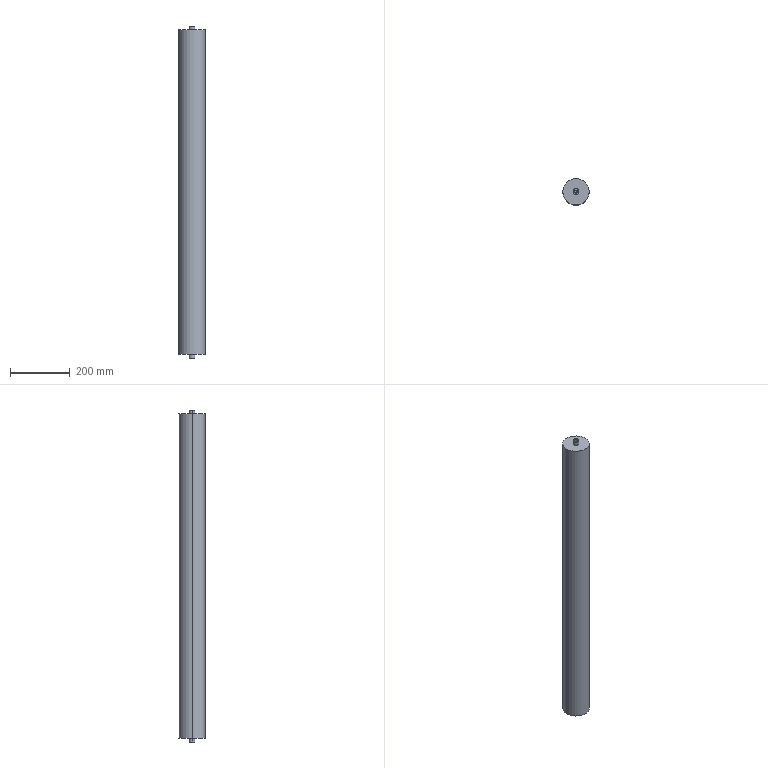Part | SolidWorks | features HoleWzd 2, ICE 2, Extrusion 1 | 1 solid | 18 faces | box 89 x 89 x 1116 mm | volume 6784916 mm3 | cylinder 10 | cone 4 | plane 4 | commonest cylinder face diameters 10.2 x4 20 x4 89 x2
STEP:
#1=CARTESIAN_POINT('',(-5.1,0.,1077.75));
#2=VERTEX_POINT('',#1);
#3=CARTESIAN_POINT('',(5.1,0.,1077.75));
#4=VERTEX_POINT('',#3);
#5=CARTESIAN_POINT('',(0.,0.,1077.75));
#6=DIRECTION('',(0.,0.,1.));
#7=DIRECTION('',(1.,0.,0.));
#8=AXIS2_PLACEMENT_3D('',#5,#6,#7);
#9=CIRCLE('',#8,5.1);
#10=EDGE_CURVE('',#2,#4,#9,.T.);
#11=ORIENTED_EDGE('',*,*,#10,.F.);
#12=CARTESIAN_POINT('',(-5.1,0.,1103.));
#13=VERTEX_POINT('',#12);
#14=CARTESIAN_POINT('',(-5.1,0.,1103.));
#15=DIRECTION('',(0.,0.,1.));
#16=VECTOR('',#15,1000.);
#17=LINE('',#14,#16);
#18=EDGE_CURVE('',#2,#13,#17,.T.);
#19=ORIENTED_EDGE('',*,*,#18,.T.);
#20=CARTESIAN_POINT('',(5.1,0.,1103.));
#21=VERTEX_POINT('',#20);
#22=CARTESIAN_POINT('',(0.,0.,1103.));
#23=DIRECTION('',(0.,0.,1.));
#24=DIRECTION('',(1.,0.,0.));
#25=AXIS2_PLACEMENT_3D('',#22,#23,#24);
#26=CIRCLE('',#25,5.1);
#27=EDGE_CURVE('',#13,#21,#26,.T.);
#28=ORIENTED_EDGE('',*,*,#27,.T.);
#29=CARTESIAN_POINT('',(5.1,0.,1103.));
#30=DIRECTION('',(0.,0.,1.));
#31=VECTOR('',#30,1000.);
#32=LINE('',#29,#31);
#33=EDGE_CURVE('',#4,#21,#32,.T.);
#34=ORIENTED_EDGE('',*,*,#33,.F.);
#35=EDGE_LOOP('',(#11,#19,#28,#34));
#36=FACE_OUTER_BOUND('',#35,.T.);
#37=CARTESIAN_POINT('',(0.,0.,1103.));
#38=DIRECTION('',(0.,0.,1.));
#39=DIRECTION('',(1.,0.,0.));
#40=AXIS2_PLACEMENT_3D('',#37,#38,#39);
#41=CYLINDRICAL_SURFACE('',#40,5.1);
#42=ADVANCED_FACE('',(#36),#41,.F.);
#43=CARTESIAN_POINT('',(0.,0.,1074.686));
#44=VERTEX_POINT('',#43);
#45=CARTESIAN_POINT('',(5.1,0.,1077.75));
#46=DIRECTION('',(0.8572,0.,0.515));
#47=VECTOR('',#46,1000.);
#48=LINE('',#45,#47);
#49=EDGE_CURVE('',#44,#4,#48,.T.);
#50=ORIENTED_EDGE('',*,*,#49,.F.);
#51=CARTESIAN_POINT('',(-5.1,0.,1077.75));
#52=DIRECTION('',(-0.8572,0.,0.515));
#53=VECTOR('',#52,1000.);
#54=LINE('',#51,#53);
#55=EDGE_CURVE('',#44,#2,#54,.T.);
#56=ORIENTED_EDGE('',*,*,#55,.T.);
#57=ORIENTED_EDGE('',*,*,#10,.T.);
#58=EDGE_LOOP('',(#50,#56,#57));
#59=FACE_OUTER_BOUND('',#58,.T.);
#60=CARTESIAN_POINT('',(0.,0.,1077.75));
#61=DIRECTION('',(0.,0.,1.));
#62=DIRECTION('',(1.,0.,0.));
#63=AXIS2_PLACEMENT_3D('',#60,#61,#62);
#64=CONICAL_SURFACE('',#63,5.1,1.03);
#65=ADVANCED_FACE('',(#59),#64,.F.);
#66=CARTESIAN_POINT('',(5.1,0.,12.25));
#67=VERTEX_POINT('',#66);
#68=CARTESIAN_POINT('',(-5.1,0.,12.25));
#69=VERTEX_POINT('',#68);
#70=CARTESIAN_POINT('',(0.,0.,12.25));
#71=DIRECTION('',(0.,0.,-1.));
#72=DIRECTION('',(-1.,0.,0.));
#73=AXIS2_PLACEMENT_3D('',#70,#71,#72);
#74=CIRCLE('',#73,5.1);
#75=EDGE_CURVE('',#67,#69,#74,.T.);
#76=ORIENTED_EDGE('',*,*,#75,.F.);
#77=CARTESIAN_POINT('',(5.1,0.,-13.));
#78=VERTEX_POINT('',#77);
#79=CARTESIAN_POINT('',(5.1,0.,-13.));
#80=DIRECTION('',(0.,0.,-1.));
#81=VECTOR('',#80,1000.);
#82=LINE('',#79,#81);
#83=EDGE_CURVE('',#67,#78,#82,.T.);
#84=ORIENTED_EDGE('',*,*,#83,.T.);
#85=CARTESIAN_POINT('',(-5.1,0.,-13.));
#86=VERTEX_POINT('',#85);
#87=CARTESIAN_POINT('',(0.,0.,-13.));
#88=DIRECTION('',(0.,0.,-1.));
#89=DIRECTION('',(-1.,0.,0.));
#90=AXIS2_PLACEMENT_3D('',#87,#88,#89);
#91=CIRCLE('',#90,5.1);
#92=EDGE_CURVE('',#78,#86,#91,.T.);
#93=ORIENTED_EDGE('',*,*,#92,.T.);
#94=CARTESIAN_POINT('',(-5.1,0.,-13.));
#95=DIRECTION('',(0.,0.,-1.));
#96=VECTOR('',#95,1000.);
#97=LINE('',#94,#96);
#98=EDGE_CURVE('',#69,#86,#97,.T.);
#99=ORIENTED_EDGE('',*,*,#98,.F.);
#100=EDGE_LOOP('',(#76,#84,#93,#99));
#101=FACE_OUTER_BOUND('',#100,.T.);
#102=CARTESIAN_POINT('',(0.,0.,-13.));
#103=DIRECTION('',(0.,0.,-1.));
#104=DIRECTION('',(-1.,0.,0.));
#105=AXIS2_PLACEMENT_3D('',#102,#103,#104);
#106=CYLINDRICAL_SURFACE('',#105,5.1);
#107=ADVANCED_FACE('',(#101),#106,.F.);
#108=CARTESIAN_POINT('',(0.,0.,15.314));
#109=VERTEX_POINT('',#108);
#110=CARTESIAN_POINT('',(-5.1,0.,12.25));
#111=DIRECTION('',(-0.8572,0.,-0.515));
#112=VECTOR('',#111,1000.);
#113=LINE('',#110,#112);
#114=EDGE_CURVE('',#109,#69,#113,.T.);
#115=ORIENTED_EDGE('',*,*,#114,.F.);
#116=CARTESIAN_POINT('',(5.1,0.,12.25));
#117=DIRECTION('',(0.8572,0.,-0.515));
#118=VECTOR('',#117,1000.);
#119=LINE('',#116,#118);
#120=EDGE_CURVE('',#109,#67,#119,.T.);
#121=ORIENTED_EDGE('',*,*,#120,.T.);
#122=ORIENTED_EDGE('',*,*,#75,.T.);
#123=EDGE_LOOP('',(#115,#121,#122));
#124=FACE_OUTER_BOUND('',#123,.T.);
#125=CARTESIAN_POINT('',(0.,0.,12.25));
#126=DIRECTION('',(0.,0.,-1.));
#127=DIRECTION('',(-1.,0.,0.));
#128=AXIS2_PLACEMENT_3D('',#125,#126,#127);
#129=CONICAL_SURFACE('',#128,5.1,1.03);
#130=ADVANCED_FACE('',(#124),#129,.F.);
#131=CARTESIAN_POINT('',(-10.,0.,-13.));
#132=VERTEX_POINT('',#131);
#133=CARTESIAN_POINT('',(10.,0.,-13.));
#134=VERTEX_POINT('',#133);
#135=CARTESIAN_POINT('',(0.,0.,-13.));
#136=DIRECTION('',(0.,0.,-1.));
#137=DIRECTION('',(-1.,0.,0.));
#138=AXIS2_PLACEMENT_3D('',#135,#136,#137);
#139=CIRCLE('',#138,10.);
#140=EDGE_CURVE('',#132,#134,#139,.T.);
#141=ORIENTED_EDGE('',*,*,#140,.F.);
#142=CARTESIAN_POINT('',(-10.,0.,0.));
#143=VERTEX_POINT('',#142);
#144=CARTESIAN_POINT('',(-10.,0.,-13.));
#145=DIRECTION('',(0.,0.,1.));
#146=VECTOR('',#145,1000.);
#147=LINE('',#144,#146);
#148=EDGE_CURVE('',#132,#143,#147,.T.);
#149=ORIENTED_EDGE('',*,*,#148,.T.);
#150=CARTESIAN_POINT('',(10.,0.,0.));
#151=VERTEX_POINT('',#150);
#152=CARTESIAN_POINT('',(0.,0.,0.));
#153=DIRECTION('',(0.,0.,-1.));
#154=DIRECTION('',(-1.,0.,0.));
#155=AXIS2_PLACEMENT_3D('',#152,#153,#154);
#156=CIRCLE('',#155,10.);
#157=EDGE_CURVE('',#143,#151,#156,.T.);
#158=ORIENTED_EDGE('',*,*,#157,.T.);
#159=CARTESIAN_POINT('',(10.,0.,-13.));
#160=DIRECTION('',(0.,0.,1.));
#161=VECTOR('',#160,1000.);
#162=LINE('',#159,#161);
#163=EDGE_CURVE('',#134,#151,#162,.T.);
#164=ORIENTED_EDGE('',*,*,#163,.F.);
#165=EDGE_LOOP('',(#141,#149,#158,#164));
#166=FACE_OUTER_BOUND('',#165,.T.);
#167=CARTESIAN_POINT('',(0.,0.,-13.));
#168=DIRECTION('',(0.,0.,1.));
#169=DIRECTION('',(1.,0.,0.));
#170=AXIS2_PLACEMENT_3D('',#167,#168,#169);
#171=CYLINDRICAL_SURFACE('',#170,10.);
#172=ADVANCED_FACE('',(#166),#171,.T.);
#173=CARTESIAN_POINT('',(10.,0.,1103.));
#174=VERTEX_POINT('',#173);
#175=CARTESIAN_POINT('',(-10.,0.,1103.));
#176=VERTEX_POINT('',#175);
#177=CARTESIAN_POINT('',(0.,0.,1103.));
#178=DIRECTION('',(0.,0.,1.));
#179=DIRECTION('',(1.,0.,0.));
#180=AXIS2_PLACEMENT_3D('',#177,#178,#179);
#181=CIRCLE('',#180,10.);
#182=EDGE_CURVE('',#174,#176,#181,.T.);
#183=ORIENTED_EDGE('',*,*,#182,.F.);
#184=CARTESIAN_POINT('',(10.,0.,1090.));
#185=VERTEX_POINT('',#184);
#186=CARTESIAN_POINT('',(10.,0.,1103.));
#187=DIRECTION('',(0.,0.,-1.));
#188=VECTOR('',#187,1000.);
#189=LINE('',#186,#188);
#190=EDGE_CURVE('',#174,#185,#189,.T.);
#191=ORIENTED_EDGE('',*,*,#190,.T.);
#192=CARTESIAN_POINT('',(-10.,0.,1090.));
#193=VERTEX_POINT('',#192);
#194=CARTESIAN_POINT('',(0.,0.,1090.));
#195=DIRECTION('',(0.,0.,1.));
#196=DIRECTION('',(1.,0.,0.));
#197=AXIS2_PLACEMENT_3D('',#194,#195,#196);
#198=CIRCLE('',#197,10.);
#199=EDGE_CURVE('',#185,#193,#198,.T.);
#200=ORIENTED_EDGE('',*,*,#199,.T.);
#201=CARTESIAN_POINT('',(-10.,0.,1103.));
#202=DIRECTION('',(0.,0.,-1.));
#203=VECTOR('',#202,1000.);
#204=LINE('',#201,#203);
#205=EDGE_CURVE('',#176,#193,#204,.T.);
#206=ORIENTED_EDGE('',*,*,#205,.F.);
#207=EDGE_LOOP('',(#183,#191,#200,#206));
#208=FACE_OUTER_BOUND('',#207,.T.);
#209=CARTESIAN_POINT('',(0.,0.,1103.));
#210=DIRECTION('',(0.,0.,-1.));
#211=DIRECTION('',(-1.,0.,0.));
#212=AXIS2_PLACEMENT_3D('',#209,#210,#211);
#213=CYLINDRICAL_SURFACE('',#212,10.);
#214=ADVANCED_FACE('',(#208),#213,.T.);
#215=CARTESIAN_POINT('',(44.5,0.,1090.));
#216=VERTEX_POINT('',#215);
#217=CARTESIAN_POINT('',(-44.5,0.,1090.));
#218=VERTEX_POINT('',#217);
#219=CARTESIAN_POINT('',(0.,0.,1090.));
#220=DIRECTION('',(0.,0.,1.));
#221=DIRECTION('',(1.,0.,0.));
#222=AXIS2_PLACEMENT_3D('',#219,#220,#221);
#223=CIRCLE('',#222,44.5);
#224=EDGE_CURVE('',#216,#218,#223,.T.);
#225=ORIENTED_EDGE('',*,*,#224,.F.);
#226=CARTESIAN_POINT('',(44.5,0.,0.));
#227=VERTEX_POINT('',#226);
#228=CARTESIAN_POINT('',(44.5,0.,1090.));
#229=DIRECTION('',(0.,0.,-1.));
#230=VECTOR('',#229,1000.);
#231=LINE('',#228,#230);
#232=EDGE_CURVE('',#216,#227,#231,.T.);
#233=ORIENTED_EDGE('',*,*,#232,.T.);
#234=CARTESIAN_POINT('',(-44.5,0.,0.));
#235=VERTEX_POINT('',#234);
#236=CARTESIAN_POINT('',(0.,0.,0.));
#237=DIRECTION('',(0.,0.,1.));
#238=DIRECTION('',(1.,0.,0.));
#239=AXIS2_PLACEMENT_3D('',#236,#237,#238);
#240=CIRCLE('',#239,44.5);
#241=EDGE_CURVE('',#227,#235,#240,.T.);
#242=ORIENTED_EDGE('',*,*,#241,.T.);
#243=CARTESIAN_POINT('',(-44.5,0.,1090.));
#244=DIRECTION('',(0.,0.,-1.));
#245=VECTOR('',#244,1000.);
#246=LINE('',#243,#245);
#247=EDGE_CURVE('',#218,#235,#246,.T.);
#248=ORIENTED_EDGE('',*,*,#247,.F.);
#249=EDGE_LOOP('',(#225,#233,#242,#248));
#250=FACE_OUTER_BOUND('',#249,.T.);
#251=CARTESIAN_POINT('',(0.,0.,1090.));
#252=DIRECTION('',(0.,0.,-1.));
#253=DIRECTION('',(-1.,0.,0.));
#254=AXIS2_PLACEMENT_3D('',#251,#252,#253);
#255=CYLINDRICAL_SURFACE('',#254,44.5);
#256=ADVANCED_FACE('',(#250),#255,.T.);
#257=ORIENTED_EDGE('',*,*,#232,.F.);
#258=CARTESIAN_POINT('',(0.,0.,1090.));
#259=DIRECTION('',(0.,0.,1.));
#260=DIRECTION('',(1.,0.,0.));
#261=AXIS2_PLACEMENT_3D('',#258,#259,#260);
#262=CIRCLE('',#261,44.5);
#263=EDGE_CURVE('',#218,#216,#262,.T.);
#264=ORIENTED_EDGE('',*,*,#263,.F.);
#265=ORIENTED_EDGE('',*,*,#247,.T.);
#266=CARTESIAN_POINT('',(0.,0.,0.));
#267=DIRECTION('',(0.,0.,1.));
#268=DIRECTION('',(1.,0.,0.));
#269=AXIS2_PLACEMENT_3D('',#266,#267,#268);
#270=CIRCLE('',#269,44.5);
#271=EDGE_CURVE('',#235,#227,#270,.T.);
#272=ORIENTED_EDGE('',*,*,#271,.T.);
#273=EDGE_LOOP('',(#257,#264,#265,#272));
#274=FACE_OUTER_BOUND('',#273,.T.);
#275=CARTESIAN_POINT('',(0.,0.,1090.));
#276=DIRECTION('',(0.,0.,-1.));
#277=DIRECTION('',(-1.,0.,0.));
#278=AXIS2_PLACEMENT_3D('',#275,#276,#277);
#279=CYLINDRICAL_SURFACE('',#278,44.5);
#280=ADVANCED_FACE('',(#274),#279,.T.);
#281=CARTESIAN_POINT('',(0.,0.,1090.));
#282=DIRECTION('',(0.,0.,1.));
#283=DIRECTION('',(1.,0.,0.));
#284=AXIS2_PLACEMENT_3D('',#281,#282,#283);
#285=CIRCLE('',#284,10.);
#286=EDGE_CURVE('',#193,#185,#285,.T.);
#287=ORIENTED_EDGE('',*,*,#286,.F.);
#288=ORIENTED_EDGE('',*,*,#199,.F.);
#289=EDGE_LOOP('',(#287,#288));
#290=FACE_BOUND('',#289,.T.);
#291=ORIENTED_EDGE('',*,*,#263,.T.);
#292=ORIENTED_EDGE('',*,*,#224,.T.);
#293=EDGE_LOOP('',(#291,#292));
#294=FACE_OUTER_BOUND('',#293,.T.);
#295=CARTESIAN_POINT('',(0.,0.,1090.));
#296=DIRECTION('',(0.,0.,1.));
#297=DIRECTION('',(1.,0.,0.));
#298=AXIS2_PLACEMENT_3D('',#295,#296,#297);
#299=PLANE('',#298);
#300=ADVANCED_FACE('',(#290,#294),#299,.T.);
#301=CARTESIAN_POINT('',(0.,0.,0.));
#302=DIRECTION('',(0.,0.,-1.));
#303=DIRECTION('',(-1.,0.,0.));
#304=AXIS2_PLACEMENT_3D('',#301,#302,#303);
#305=CIRCLE('',#304,10.);
#306=EDGE_CURVE('',#151,#143,#305,.T.);
#307=ORIENTED_EDGE('',*,*,#306,.F.);
#308=ORIENTED_EDGE('',*,*,#157,.F.);
#309=EDGE_LOOP('',(#307,#308));
#310=FACE_BOUND('',#309,.T.);
#311=ORIENTED_EDGE('',*,*,#271,.F.);
#312=ORIENTED_EDGE('',*,*,#241,.F.);
#313=EDGE_LOOP('',(#311,#312));
#314=FACE_OUTER_BOUND('',#313,.T.);
#315=CARTESIAN_POINT('',(0.,0.,0.));
#316=DIRECTION('',(0.,0.,1.));
#317=DIRECTION('',(1.,0.,0.));
#318=AXIS2_PLACEMENT_3D('',#315,#316,#317);
#319=PLANE('',#318);
#320=ADVANCED_FACE('',(#310,#314),#319,.F.);
#321=ORIENTED_EDGE('',*,*,#190,.F.);
#322=CARTESIAN_POINT('',(0.,0.,1103.));
#323=DIRECTION('',(0.,0.,1.));
#324=DIRECTION('',(1.,0.,0.));
#325=AXIS2_PLACEMENT_3D('',#322,#323,#324);
#326=CIRCLE('',#325,10.);
#327=EDGE_CURVE('',#176,#174,#326,.T.);
#328=ORIENTED_EDGE('',*,*,#327,.F.);
#329=ORIENTED_EDGE('',*,*,#205,.T.);
#330=ORIENTED_EDGE('',*,*,#286,.T.);
#331=EDGE_LOOP('',(#321,#328,#329,#330));
#332=FACE_OUTER_BOUND('',#331,.T.);
#333=CARTESIAN_POINT('',(0.,0.,1103.));
#334=DIRECTION('',(0.,0.,-1.));
#335=DIRECTION('',(-1.,0.,0.));
#336=AXIS2_PLACEMENT_3D('',#333,#334,#335);
#337=CYLINDRICAL_SURFACE('',#336,10.);
#338=ADVANCED_FACE('',(#332),#337,.T.);
#339=CARTESIAN_POINT('',(0.,0.,1103.));
#340=DIRECTION('',(0.,0.,1.));
#341=DIRECTION('',(1.,0.,0.));
#342=AXIS2_PLACEMENT_3D('',#339,#340,#341);
#343=CIRCLE('',#342,5.1);
#344=EDGE_CURVE('',#21,#13,#343,.T.);
#345=ORIENTED_EDGE('',*,*,#344,.F.);
#346=ORIENTED_EDGE('',*,*,#27,.F.);
#347=EDGE_LOOP('',(#345,#346));
#348=FACE_BOUND('',#347,.T.);
#349=ORIENTED_EDGE('',*,*,#327,.T.);
#350=ORIENTED_EDGE('',*,*,#182,.T.);
#351=EDGE_LOOP('',(#349,#350));
#352=FACE_OUTER_BOUND('',#351,.T.);
#353=CARTESIAN_POINT('',(0.,0.,1103.));
#354=DIRECTION('',(0.,0.,1.));
#355=DIRECTION('',(1.,0.,0.));
#356=AXIS2_PLACEMENT_3D('',#353,#354,#355);
#357=PLANE('',#356);
#358=ADVANCED_FACE('',(#348,#352),#357,.T.);
#359=ORIENTED_EDGE('',*,*,#148,.F.);
#360=CARTESIAN_POINT('',(0.,0.,-13.));
#361=DIRECTION('',(0.,0.,-1.));
#362=DIRECTION('',(-1.,0.,0.));
#363=AXIS2_PLACEMENT_3D('',#360,#361,#362);
#364=CIRCLE('',#363,10.);
#365=EDGE_CURVE('',#134,#132,#364,.T.);
#366=ORIENTED_EDGE('',*,*,#365,.F.);
#367=ORIENTED_EDGE('',*,*,#163,.T.);
#368=ORIENTED_EDGE('',*,*,#306,.T.);
#369=EDGE_LOOP('',(#359,#366,#367,#368));
#370=FACE_OUTER_BOUND('',#369,.T.);
#371=CARTESIAN_POINT('',(0.,0.,-13.));
#372=DIRECTION('',(0.,0.,1.));
#373=DIRECTION('',(1.,0.,0.));
#374=AXIS2_PLACEMENT_3D('',#371,#372,#373);
#375=CYLINDRICAL_SURFACE('',#374,10.);
#376=ADVANCED_FACE('',(#370),#375,.T.);
#377=CARTESIAN_POINT('',(0.,0.,-13.));
#378=DIRECTION('',(0.,0.,-1.));
#379=DIRECTION('',(-1.,0.,0.));
#380=AXIS2_PLACEMENT_3D('',#377,#378,#379);
#381=CIRCLE('',#380,5.1);
#382=EDGE_CURVE('',#86,#78,#381,.T.);
#383=ORIENTED_EDGE('',*,*,#382,.F.);
#384=ORIENTED_EDGE('',*,*,#92,.F.);
#385=EDGE_LOOP('',(#383,#384));
#386=FACE_BOUND('',#385,.T.);
#387=ORIENTED_EDGE('',*,*,#365,.T.);
#388=ORIENTED_EDGE('',*,*,#140,.T.);
#389=EDGE_LOOP('',(#387,#388));
#390=FACE_OUTER_BOUND('',#389,.T.);
#391=CARTESIAN_POINT('',(0.,0.,-13.));
#392=DIRECTION('',(0.,0.,-1.));
#393=DIRECTION('',(-1.,0.,0.));
#394=AXIS2_PLACEMENT_3D('',#391,#392,#393);
#395=PLANE('',#394);
#396=ADVANCED_FACE('',(#386,#390),#395,.T.);
#397=ORIENTED_EDGE('',*,*,#120,.F.);
#398=ORIENTED_EDGE('',*,*,#114,.T.);
#399=CARTESIAN_POINT('',(0.,0.,12.25));
#400=DIRECTION('',(0.,0.,-1.));
#401=DIRECTION('',(-1.,0.,0.));
#402=AXIS2_PLACEMENT_3D('',#399,#400,#401);
#403=CIRCLE('',#402,5.1);
#404=EDGE_CURVE('',#69,#67,#403,.T.);
#405=ORIENTED_EDGE('',*,*,#404,.T.);
#406=EDGE_LOOP('',(#397,#398,#405));
#407=FACE_OUTER_BOUND('',#406,.T.);
#408=CARTESIAN_POINT('',(0.,0.,12.25));
#409=DIRECTION('',(0.,0.,-1.));
#410=DIRECTION('',(-1.,0.,0.));
#411=AXIS2_PLACEMENT_3D('',#408,#409,#410);
#412=CONICAL_SURFACE('',#411,5.1,1.03);
#413=ADVANCED_FACE('',(#407),#412,.F.);
#414=ORIENTED_EDGE('',*,*,#83,.F.);
#415=ORIENTED_EDGE('',*,*,#404,.F.);
#416=ORIENTED_EDGE('',*,*,#98,.T.);
#417=ORIENTED_EDGE('',*,*,#382,.T.);
#418=EDGE_LOOP('',(#414,#415,#416,#417));
#419=FACE_OUTER_BOUND('',#418,.T.);
#420=CARTESIAN_POINT('',(0.,0.,-13.));
#421=DIRECTION('',(0.,0.,-1.));
#422=DIRECTION('',(-1.,0.,0.));
#423=AXIS2_PLACEMENT_3D('',#420,#421,#422);
#424=CYLINDRICAL_SURFACE('',#423,5.1);
#425=ADVANCED_FACE('',(#419),#424,.F.);
#426=ORIENTED_EDGE('',*,*,#55,.F.);
#427=ORIENTED_EDGE('',*,*,#49,.T.);
#428=CARTESIAN_POINT('',(0.,0.,1077.75));
#429=DIRECTION('',(0.,0.,1.));
#430=DIRECTION('',(1.,0.,0.));
#431=AXIS2_PLACEMENT_3D('',#428,#429,#430);
#432=CIRCLE('',#431,5.1);
#433=EDGE_CURVE('',#4,#2,#432,.T.);
#434=ORIENTED_EDGE('',*,*,#433,.T.);
#435=EDGE_LOOP('',(#426,#427,#434));
#436=FACE_OUTER_BOUND('',#435,.T.);
#437=CARTESIAN_POINT('',(0.,0.,1077.75));
#438=DIRECTION('',(0.,0.,1.));
#439=DIRECTION('',(1.,0.,0.));
#440=AXIS2_PLACEMENT_3D('',#437,#438,#439);
#441=CONICAL_SURFACE('',#440,5.1,1.03);
#442=ADVANCED_FACE('',(#436),#441,.F.);
#443=ORIENTED_EDGE('',*,*,#18,.F.);
#444=ORIENTED_EDGE('',*,*,#433,.F.);
#445=ORIENTED_EDGE('',*,*,#33,.T.);
#446=ORIENTED_EDGE('',*,*,#344,.T.);
#447=EDGE_LOOP('',(#443,#444,#445,#446));
#448=FACE_OUTER_BOUND('',#447,.T.);
#449=CARTESIAN_POINT('',(0.,0.,1103.));
#450=DIRECTION('',(0.,0.,1.));
#451=DIRECTION('',(1.,0.,0.));
#452=AXIS2_PLACEMENT_3D('',#449,#450,#451);
#453=CYLINDRICAL_SURFACE('',#452,5.1);
#454=ADVANCED_FACE('',(#448),#453,.F.);
#455=CLOSED_SHELL('',(#42,#65,#107,#130,#172,#214,#256,#280,#300,#320,#338,#358,#376,#396,#413,#425,#442,#454));
#456=MANIFOLD_SOLID_BREP('',#455);
#457=CARTESIAN_POINT('',(0.,0.,0.));
#458=DIRECTION('',(0.,0.,1.));
#459=DIRECTION('',(1.,0.,0.));
#460=AXIS2_PLACEMENT_3D('',#457,#458,#459);
#461=(LENGTH_UNIT()NAMED_UNIT(*)SI_UNIT(.MILLI.,.METRE.));
#462=UNCERTAINTY_MEASURE_WITH_UNIT(LENGTH_MEASURE(0.00001),#461,'','');
#463=(NAMED_UNIT(*)PLANE_ANGLE_UNIT()SI_UNIT($,.RADIAN.));
#464=(NAMED_UNIT(*)SI_UNIT($,.STERADIAN.)SOLID_ANGLE_UNIT());
#465=(GEOMETRIC_REPRESENTATION_CONTEXT(3)GLOBAL_UNCERTAINTY_ASSIGNED_CONTEXT((#462))GLOBAL_UNIT_ASSIGNED_CONTEXT((#461,#463,#464))REPRESENTATION_CONTEXT('',''));
#466=ADVANCED_BREP_SHAPE_REPRESENTATION('',(#456,#460),#465);